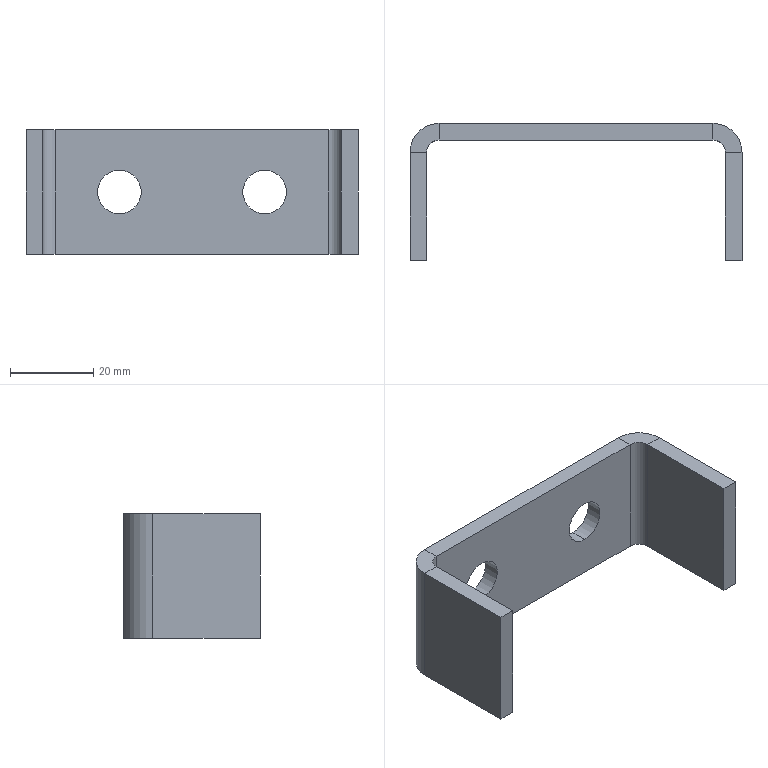Part | STEP file | SYL_0392D6J1SYL0380DJ10-1609202 | 1 solid | 26 faces | box 80 x 33 x 30 mm | volume 15352 mm3 | plane 18 | cylinder 8 | commonest cylinder face diameters 10.5 x4 6 x2 14 x2
STEP:
#1=CARTESIAN_POINT('',(-17.5,4.,5.25));
#2=VERTEX_POINT('',#1);
#3=CARTESIAN_POINT('',(-17.5,0.,5.25));
#4=VERTEX_POINT('',#3);
#5=CARTESIAN_POINT('',(-17.5,0.,5.25));
#6=DIRECTION('',(0.,-1.,0.));
#7=VECTOR('',#6,1000.);
#8=LINE('',#5,#7);
#9=EDGE_CURVE('',#2,#4,#8,.T.);
#10=ORIENTED_EDGE('',*,*,#9,.F.);
#11=CARTESIAN_POINT('',(-17.5,4.,-5.25));
#12=VERTEX_POINT('',#11);
#13=CARTESIAN_POINT('',(-17.5,4.,0.));
#14=DIRECTION('',(0.,1.,0.));
#15=DIRECTION('',(0.,0.,1.));
#16=AXIS2_PLACEMENT_3D('',#13,#14,#15);
#17=CIRCLE('',#16,5.25);
#18=EDGE_CURVE('',#2,#12,#17,.T.);
#19=ORIENTED_EDGE('',*,*,#18,.T.);
#20=CARTESIAN_POINT('',(-17.5,0.,-5.25));
#21=VERTEX_POINT('',#20);
#22=CARTESIAN_POINT('',(-17.5,0.,-5.25));
#23=DIRECTION('',(0.,-1.,0.));
#24=VECTOR('',#23,1000.);
#25=LINE('',#22,#24);
#26=EDGE_CURVE('',#12,#21,#25,.T.);
#27=ORIENTED_EDGE('',*,*,#26,.T.);
#28=CARTESIAN_POINT('',(-17.5,0.,0.));
#29=DIRECTION('',(0.,1.,0.));
#30=DIRECTION('',(0.,0.,1.));
#31=AXIS2_PLACEMENT_3D('',#28,#29,#30);
#32=CIRCLE('',#31,5.25);
#33=EDGE_CURVE('',#4,#21,#32,.T.);
#34=ORIENTED_EDGE('',*,*,#33,.F.);
#35=EDGE_LOOP('',(#10,#19,#27,#34));
#36=FACE_OUTER_BOUND('',#35,.T.);
#37=CARTESIAN_POINT('',(-17.5,0.,0.));
#38=DIRECTION('',(0.,1.,0.));
#39=DIRECTION('',(0.,0.,1.));
#40=AXIS2_PLACEMENT_3D('',#37,#38,#39);
#41=CYLINDRICAL_SURFACE('',#40,5.25);
#42=ADVANCED_FACE('',(#36),#41,.F.);
#43=CARTESIAN_POINT('',(17.5,4.,5.25));
#44=VERTEX_POINT('',#43);
#45=CARTESIAN_POINT('',(17.5,0.,5.25));
#46=VERTEX_POINT('',#45);
#47=CARTESIAN_POINT('',(17.5,0.,5.25));
#48=DIRECTION('',(0.,-1.,0.));
#49=VECTOR('',#48,1000.);
#50=LINE('',#47,#49);
#51=EDGE_CURVE('',#44,#46,#50,.T.);
#52=ORIENTED_EDGE('',*,*,#51,.F.);
#53=CARTESIAN_POINT('',(17.5,4.,-5.25));
#54=VERTEX_POINT('',#53);
#55=CARTESIAN_POINT('',(17.5,4.,0.));
#56=DIRECTION('',(0.,1.,0.));
#57=DIRECTION('',(0.,0.,1.));
#58=AXIS2_PLACEMENT_3D('',#55,#56,#57);
#59=CIRCLE('',#58,5.25);
#60=EDGE_CURVE('',#44,#54,#59,.T.);
#61=ORIENTED_EDGE('',*,*,#60,.T.);
#62=CARTESIAN_POINT('',(17.5,0.,-5.25));
#63=VERTEX_POINT('',#62);
#64=CARTESIAN_POINT('',(17.5,0.,-5.25));
#65=DIRECTION('',(0.,-1.,0.));
#66=VECTOR('',#65,1000.);
#67=LINE('',#64,#66);
#68=EDGE_CURVE('',#54,#63,#67,.T.);
#69=ORIENTED_EDGE('',*,*,#68,.T.);
#70=CARTESIAN_POINT('',(17.5,0.,0.));
#71=DIRECTION('',(0.,1.,0.));
#72=DIRECTION('',(0.,0.,1.));
#73=AXIS2_PLACEMENT_3D('',#70,#71,#72);
#74=CIRCLE('',#73,5.25);
#75=EDGE_CURVE('',#46,#63,#74,.T.);
#76=ORIENTED_EDGE('',*,*,#75,.F.);
#77=EDGE_LOOP('',(#52,#61,#69,#76));
#78=FACE_OUTER_BOUND('',#77,.T.);
#79=CARTESIAN_POINT('',(17.5,0.,0.));
#80=DIRECTION('',(0.,1.,0.));
#81=DIRECTION('',(0.,0.,1.));
#82=AXIS2_PLACEMENT_3D('',#79,#80,#81);
#83=CYLINDRICAL_SURFACE('',#82,5.25);
#84=ADVANCED_FACE('',(#78),#83,.F.);
#85=CARTESIAN_POINT('',(40.,-29.,-15.));
#86=VERTEX_POINT('',#85);
#87=CARTESIAN_POINT('',(36.,-29.,-15.));
#88=VERTEX_POINT('',#87);
#89=CARTESIAN_POINT('',(36.,-29.,-15.));
#90=DIRECTION('',(-1.,0.,0.));
#91=VECTOR('',#90,1000.);
#92=LINE('',#89,#91);
#93=EDGE_CURVE('',#86,#88,#92,.T.);
#94=ORIENTED_EDGE('',*,*,#93,.F.);
#95=CARTESIAN_POINT('',(40.,-29.,15.));
#96=VERTEX_POINT('',#95);
#97=CARTESIAN_POINT('',(40.,-29.,15.));
#98=DIRECTION('',(0.,0.,1.));
#99=VECTOR('',#98,1000.);
#100=LINE('',#97,#99);
#101=EDGE_CURVE('',#86,#96,#100,.T.);
#102=ORIENTED_EDGE('',*,*,#101,.T.);
#103=CARTESIAN_POINT('',(36.,-29.,15.));
#104=VERTEX_POINT('',#103);
#105=CARTESIAN_POINT('',(36.,-29.,15.));
#106=DIRECTION('',(-1.,0.,0.));
#107=VECTOR('',#106,1000.);
#108=LINE('',#105,#107);
#109=EDGE_CURVE('',#96,#104,#108,.T.);
#110=ORIENTED_EDGE('',*,*,#109,.T.);
#111=CARTESIAN_POINT('',(36.,-29.,-15.));
#112=DIRECTION('',(0.,0.,1.));
#113=VECTOR('',#112,1000.);
#114=LINE('',#111,#113);
#115=EDGE_CURVE('',#88,#104,#114,.T.);
#116=ORIENTED_EDGE('',*,*,#115,.F.);
#117=EDGE_LOOP('',(#94,#102,#110,#116));
#118=FACE_OUTER_BOUND('',#117,.T.);
#119=CARTESIAN_POINT('',(36.,-29.,-15.));
#120=DIRECTION('',(0.,1.,0.));
#121=DIRECTION('',(0.,0.,1.));
#122=AXIS2_PLACEMENT_3D('',#119,#120,#121);
#123=PLANE('',#122);
#124=ADVANCED_FACE('',(#118),#123,.F.);
#125=ORIENTED_EDGE('',*,*,#109,.F.);
#126=CARTESIAN_POINT('',(40.,-3.,15.));
#127=VERTEX_POINT('',#126);
#128=CARTESIAN_POINT('',(40.,4.,15.));
#129=DIRECTION('',(0.,1.,0.));
#130=VECTOR('',#129,1000.);
#131=LINE('',#128,#130);
#132=EDGE_CURVE('',#96,#127,#131,.T.);
#133=ORIENTED_EDGE('',*,*,#132,.T.);
#134=CARTESIAN_POINT('',(36.,-3.,15.));
#135=VERTEX_POINT('',#134);
#136=CARTESIAN_POINT('',(36.,-3.,15.));
#137=DIRECTION('',(-1.,0.,0.));
#138=VECTOR('',#137,1000.);
#139=LINE('',#136,#138);
#140=EDGE_CURVE('',#127,#135,#139,.T.);
#141=ORIENTED_EDGE('',*,*,#140,.T.);
#142=CARTESIAN_POINT('',(36.,-29.,15.));
#143=DIRECTION('',(0.,1.,0.));
#144=VECTOR('',#143,1000.);
#145=LINE('',#142,#144);
#146=EDGE_CURVE('',#104,#135,#145,.T.);
#147=ORIENTED_EDGE('',*,*,#146,.F.);
#148=EDGE_LOOP('',(#125,#133,#141,#147));
#149=FACE_OUTER_BOUND('',#148,.T.);
#150=CARTESIAN_POINT('',(36.,-29.,15.));
#151=DIRECTION('',(0.,0.,-1.));
#152=DIRECTION('',(0.,1.,0.));
#153=AXIS2_PLACEMENT_3D('',#150,#151,#152);
#154=PLANE('',#153);
#155=ADVANCED_FACE('',(#149),#154,.F.);
#156=ORIENTED_EDGE('',*,*,#140,.F.);
#157=CARTESIAN_POINT('',(33.,4.,15.));
#158=VERTEX_POINT('',#157);
#159=CARTESIAN_POINT('',(33.,-3.,15.));
#160=DIRECTION('',(0.,0.,-1.));
#161=DIRECTION('',(1.,0.,0.));
#162=AXIS2_PLACEMENT_3D('',#159,#160,#161);
#163=CIRCLE('',#162,7.);
#164=EDGE_CURVE('',#158,#127,#163,.T.);
#165=ORIENTED_EDGE('',*,*,#164,.F.);
#166=CARTESIAN_POINT('',(33.,0.,15.));
#167=VERTEX_POINT('',#166);
#168=CARTESIAN_POINT('',(33.,0.,15.));
#169=DIRECTION('',(0.,-1.,0.));
#170=VECTOR('',#169,1000.);
#171=LINE('',#168,#170);
#172=EDGE_CURVE('',#158,#167,#171,.T.);
#173=ORIENTED_EDGE('',*,*,#172,.T.);
#174=CARTESIAN_POINT('',(33.,-3.,15.));
#175=DIRECTION('',(0.,0.,-1.));
#176=DIRECTION('',(0.,1.,0.));
#177=AXIS2_PLACEMENT_3D('',#174,#175,#176);
#178=CIRCLE('',#177,3.);
#179=EDGE_CURVE('',#167,#135,#178,.T.);
#180=ORIENTED_EDGE('',*,*,#179,.T.);
#181=EDGE_LOOP('',(#156,#165,#173,#180));
#182=FACE_OUTER_BOUND('',#181,.T.);
#183=CARTESIAN_POINT('',(33.,-3.,15.));
#184=DIRECTION('',(0.,0.,1.));
#185=DIRECTION('',(1.,0.,0.));
#186=AXIS2_PLACEMENT_3D('',#183,#184,#185);
#187=PLANE('',#186);
#188=ADVANCED_FACE('',(#182),#187,.T.);
#189=ORIENTED_EDGE('',*,*,#172,.F.);
#190=CARTESIAN_POINT('',(-33.,4.,15.));
#191=VERTEX_POINT('',#190);
#192=CARTESIAN_POINT('',(0.,4.,15.));
#193=DIRECTION('',(-1.,0.,0.));
#194=VECTOR('',#193,1000.);
#195=LINE('',#192,#194);
#196=EDGE_CURVE('',#158,#191,#195,.T.);
#197=ORIENTED_EDGE('',*,*,#196,.T.);
#198=CARTESIAN_POINT('',(-33.,0.,15.));
#199=VERTEX_POINT('',#198);
#200=CARTESIAN_POINT('',(-33.,0.,15.));
#201=DIRECTION('',(0.,-1.,0.));
#202=VECTOR('',#201,1000.);
#203=LINE('',#200,#202);
#204=EDGE_CURVE('',#191,#199,#203,.T.);
#205=ORIENTED_EDGE('',*,*,#204,.T.);
#206=CARTESIAN_POINT('',(33.,0.,15.));
#207=DIRECTION('',(-1.,0.,0.));
#208=VECTOR('',#207,1000.);
#209=LINE('',#206,#208);
#210=EDGE_CURVE('',#167,#199,#209,.T.);
#211=ORIENTED_EDGE('',*,*,#210,.F.);
#212=EDGE_LOOP('',(#189,#197,#205,#211));
#213=FACE_OUTER_BOUND('',#212,.T.);
#214=CARTESIAN_POINT('',(33.,0.,15.));
#215=DIRECTION('',(0.,0.,-1.));
#216=DIRECTION('',(-1.,0.,0.));
#217=AXIS2_PLACEMENT_3D('',#214,#215,#216);
#218=PLANE('',#217);
#219=ADVANCED_FACE('',(#213),#218,.F.);
#220=ORIENTED_EDGE('',*,*,#204,.F.);
#221=CARTESIAN_POINT('',(-40.,-3.,15.));
#222=VERTEX_POINT('',#221);
#223=CARTESIAN_POINT('',(-33.,-3.,15.));
#224=DIRECTION('',(0.,0.,-1.));
#225=DIRECTION('',(-1.,0.,0.));
#226=AXIS2_PLACEMENT_3D('',#223,#224,#225);
#227=CIRCLE('',#226,7.);
#228=EDGE_CURVE('',#222,#191,#227,.T.);
#229=ORIENTED_EDGE('',*,*,#228,.F.);
#230=CARTESIAN_POINT('',(-36.,-3.,15.));
#231=VERTEX_POINT('',#230);
#232=CARTESIAN_POINT('',(-36.,-3.,15.));
#233=DIRECTION('',(1.,0.,0.));
#234=VECTOR('',#233,1000.);
#235=LINE('',#232,#234);
#236=EDGE_CURVE('',#222,#231,#235,.T.);
#237=ORIENTED_EDGE('',*,*,#236,.T.);
#238=CARTESIAN_POINT('',(-33.,-3.,15.));
#239=DIRECTION('',(0.,0.,-1.));
#240=DIRECTION('',(-1.,0.,0.));
#241=AXIS2_PLACEMENT_3D('',#238,#239,#240);
#242=CIRCLE('',#241,3.);
#243=EDGE_CURVE('',#231,#199,#242,.T.);
#244=ORIENTED_EDGE('',*,*,#243,.T.);
#245=EDGE_LOOP('',(#220,#229,#237,#244));
#246=FACE_OUTER_BOUND('',#245,.T.);
#247=CARTESIAN_POINT('',(-33.,-3.,15.));
#248=DIRECTION('',(0.,0.,1.));
#249=DIRECTION('',(1.,0.,0.));
#250=AXIS2_PLACEMENT_3D('',#247,#248,#249);
#251=PLANE('',#250);
#252=ADVANCED_FACE('',(#246),#251,.T.);
#253=ORIENTED_EDGE('',*,*,#236,.F.);
#254=CARTESIAN_POINT('',(-40.,-29.,15.));
#255=VERTEX_POINT('',#254);
#256=CARTESIAN_POINT('',(-40.,4.,15.));
#257=DIRECTION('',(0.,-1.,0.));
#258=VECTOR('',#257,1000.);
#259=LINE('',#256,#258);
#260=EDGE_CURVE('',#222,#255,#259,.T.);
#261=ORIENTED_EDGE('',*,*,#260,.T.);
#262=CARTESIAN_POINT('',(-36.,-29.,15.));
#263=VERTEX_POINT('',#262);
#264=CARTESIAN_POINT('',(-36.,-29.,15.));
#265=DIRECTION('',(1.,0.,0.));
#266=VECTOR('',#265,1000.);
#267=LINE('',#264,#266);
#268=EDGE_CURVE('',#255,#263,#267,.T.);
#269=ORIENTED_EDGE('',*,*,#268,.T.);
#270=CARTESIAN_POINT('',(-36.,-3.,15.));
#271=DIRECTION('',(0.,-1.,0.));
#272=VECTOR('',#271,1000.);
#273=LINE('',#270,#272);
#274=EDGE_CURVE('',#231,#263,#273,.T.);
#275=ORIENTED_EDGE('',*,*,#274,.F.);
#276=EDGE_LOOP('',(#253,#261,#269,#275));
#277=FACE_OUTER_BOUND('',#276,.T.);
#278=CARTESIAN_POINT('',(-36.,-3.,15.));
#279=DIRECTION('',(0.,0.,-1.));
#280=DIRECTION('',(0.,-1.,0.));
#281=AXIS2_PLACEMENT_3D('',#278,#279,#280);
#282=PLANE('',#281);
#283=ADVANCED_FACE('',(#277),#282,.F.);
#284=ORIENTED_EDGE('',*,*,#268,.F.);
#285=CARTESIAN_POINT('',(-40.,-29.,-15.));
#286=VERTEX_POINT('',#285);
#287=CARTESIAN_POINT('',(-40.,-29.,-15.));
#288=DIRECTION('',(0.,0.,-1.));
#289=VECTOR('',#288,1000.);
#290=LINE('',#287,#289);
#291=EDGE_CURVE('',#255,#286,#290,.T.);
#292=ORIENTED_EDGE('',*,*,#291,.T.);
#293=CARTESIAN_POINT('',(-36.,-29.,-15.));
#294=VERTEX_POINT('',#293);
#295=CARTESIAN_POINT('',(-36.,-29.,-15.));
#296=DIRECTION('',(1.,0.,0.));
#297=VECTOR('',#296,1000.);
#298=LINE('',#295,#297);
#299=EDGE_CURVE('',#286,#294,#298,.T.);
#300=ORIENTED_EDGE('',*,*,#299,.T.);
#301=CARTESIAN_POINT('',(-36.,-29.,15.));
#302=DIRECTION('',(0.,0.,-1.));
#303=VECTOR('',#302,1000.);
#304=LINE('',#301,#303);
#305=EDGE_CURVE('',#263,#294,#304,.T.);
#306=ORIENTED_EDGE('',*,*,#305,.F.);
#307=EDGE_LOOP('',(#284,#292,#300,#306));
#308=FACE_OUTER_BOUND('',#307,.T.);
#309=CARTESIAN_POINT('',(-36.,-29.,15.));
#310=DIRECTION('',(0.,1.,0.));
#311=DIRECTION('',(0.,0.,-1.));
#312=AXIS2_PLACEMENT_3D('',#309,#310,#311);
#313=PLANE('',#312);
#314=ADVANCED_FACE('',(#308),#313,.F.);
#315=ORIENTED_EDGE('',*,*,#299,.F.);
#316=CARTESIAN_POINT('',(-40.,-3.,-15.));
#317=VERTEX_POINT('',#316);
#318=CARTESIAN_POINT('',(-40.,4.,-15.));
#319=DIRECTION('',(0.,1.,0.));
#320=VECTOR('',#319,1000.);
#321=LINE('',#318,#320);
#322=EDGE_CURVE('',#286,#317,#321,.T.);
#323=ORIENTED_EDGE('',*,*,#322,.T.);
#324=CARTESIAN_POINT('',(-36.,-3.,-15.));
#325=VERTEX_POINT('',#324);
#326=CARTESIAN_POINT('',(-36.,-3.,-15.));
#327=DIRECTION('',(1.,0.,0.));
#328=VECTOR('',#327,1000.);
#329=LINE('',#326,#328);
#330=EDGE_CURVE('',#317,#325,#329,.T.);
#331=ORIENTED_EDGE('',*,*,#330,.T.);
#332=CARTESIAN_POINT('',(-36.,-29.,-15.));
#333=DIRECTION('',(0.,1.,0.));
#334=VECTOR('',#333,1000.);
#335=LINE('',#332,#334);
#336=EDGE_CURVE('',#294,#325,#335,.T.);
#337=ORIENTED_EDGE('',*,*,#336,.F.);
#338=EDGE_LOOP('',(#315,#323,#331,#337));
#339=FACE_OUTER_BOUND('',#338,.T.);
#340=CARTESIAN_POINT('',(-36.,-29.,-15.));
#341=DIRECTION('',(0.,0.,1.));
#342=DIRECTION('',(0.,1.,0.));
#343=AXIS2_PLACEMENT_3D('',#340,#341,#342);
#344=PLANE('',#343);
#345=ADVANCED_FACE('',(#339),#344,.F.);
#346=ORIENTED_EDGE('',*,*,#330,.F.);
#347=CARTESIAN_POINT('',(-33.,4.,-15.));
#348=VERTEX_POINT('',#347);
#349=CARTESIAN_POINT('',(-33.,-3.,-15.));
#350=DIRECTION('',(0.,0.,1.));
#351=DIRECTION('',(-1.,0.,0.));
#352=AXIS2_PLACEMENT_3D('',#349,#350,#351);
#353=CIRCLE('',#352,7.);
#354=EDGE_CURVE('',#348,#317,#353,.T.);
#355=ORIENTED_EDGE('',*,*,#354,.F.);
#356=CARTESIAN_POINT('',(-33.,0.,-15.));
#357=VERTEX_POINT('',#356);
#358=CARTESIAN_POINT('',(-33.,0.,-15.));
#359=DIRECTION('',(0.,-1.,0.));
#360=VECTOR('',#359,1000.);
#361=LINE('',#358,#360);
#362=EDGE_CURVE('',#348,#357,#361,.T.);
#363=ORIENTED_EDGE('',*,*,#362,.T.);
#364=CARTESIAN_POINT('',(-33.,-3.,-15.));
#365=DIRECTION('',(0.,0.,1.));
#366=DIRECTION('',(0.,1.,0.));
#367=AXIS2_PLACEMENT_3D('',#364,#365,#366);
#368=CIRCLE('',#367,3.);
#369=EDGE_CURVE('',#357,#325,#368,.T.);
#370=ORIENTED_EDGE('',*,*,#369,.T.);
#371=EDGE_LOOP('',(#346,#355,#363,#370));
#372=FACE_OUTER_BOUND('',#371,.T.);
#373=CARTESIAN_POINT('',(-33.,-3.,-15.));
#374=DIRECTION('',(0.,0.,-1.));
#375=DIRECTION('',(-1.,0.,0.));
#376=AXIS2_PLACEMENT_3D('',#373,#374,#375);
#377=PLANE('',#376);
#378=ADVANCED_FACE('',(#372),#377,.T.);
#379=ORIENTED_EDGE('',*,*,#362,.F.);
#380=CARTESIAN_POINT('',(33.,4.,-15.));
#381=VERTEX_POINT('',#380);
#382=CARTESIAN_POINT('',(0.,4.,-15.));
#383=DIRECTION('',(1.,0.,0.));
#384=VECTOR('',#383,1000.);
#385=LINE('',#382,#384);
#386=EDGE_CURVE('',#348,#381,#385,.T.);
#387=ORIENTED_EDGE('',*,*,#386,.T.);
#388=CARTESIAN_POINT('',(33.,0.,-15.));
#389=VERTEX_POINT('',#388);
#390=CARTESIAN_POINT('',(33.,0.,-15.));
#391=DIRECTION('',(0.,-1.,0.));
#392=VECTOR('',#391,1000.);
#393=LINE('',#390,#392);
#394=EDGE_CURVE('',#381,#389,#393,.T.);
#395=ORIENTED_EDGE('',*,*,#394,.T.);
#396=CARTESIAN_POINT('',(-33.,0.,-15.));
#397=DIRECTION('',(1.,0.,0.));
#398=VECTOR('',#397,1000.);
#399=LINE('',#396,#398);
#400=EDGE_CURVE('',#357,#389,#399,.T.);
#401=ORIENTED_EDGE('',*,*,#400,.F.);
#402=EDGE_LOOP('',(#379,#387,#395,#401));
#403=FACE_OUTER_BOUND('',#402,.T.);
#404=CARTESIAN_POINT('',(-33.,0.,-15.));
#405=DIRECTION('',(0.,0.,1.));
#406=DIRECTION('',(1.,0.,0.));
#407=AXIS2_PLACEMENT_3D('',#404,#405,#406);
#408=PLANE('',#407);
#409=ADVANCED_FACE('',(#403),#408,.F.);
#410=ORIENTED_EDGE('',*,*,#394,.F.);
#411=CARTESIAN_POINT('',(40.,-3.,-15.));
#412=VERTEX_POINT('',#411);
#413=CARTESIAN_POINT('',(33.,-3.,-15.));
#414=DIRECTION('',(0.,0.,1.));
#415=DIRECTION('',(1.,0.,0.));
#416=AXIS2_PLACEMENT_3D('',#413,#414,#415);
#417=CIRCLE('',#416,7.);
#418=EDGE_CURVE('',#412,#381,#417,.T.);
#419=ORIENTED_EDGE('',*,*,#418,.F.);
#420=CARTESIAN_POINT('',(36.,-3.,-15.));
#421=VERTEX_POINT('',#420);
#422=CARTESIAN_POINT('',(36.,-3.,-15.));
#423=DIRECTION('',(-1.,0.,0.));
#424=VECTOR('',#423,1000.);
#425=LINE('',#422,#424);
#426=EDGE_CURVE('',#412,#421,#425,.T.);
#427=ORIENTED_EDGE('',*,*,#426,.T.);
#428=CARTESIAN_POINT('',(33.,-3.,-15.));
#429=DIRECTION('',(0.,0.,1.));
#430=DIRECTION('',(1.,0.,0.));
#431=AXIS2_PLACEMENT_3D('',#428,#429,#430);
#432=CIRCLE('',#431,3.);
#433=EDGE_CURVE('',#421,#389,#432,.T.);
#434=ORIENTED_EDGE('',*,*,#433,.T.);
#435=EDGE_LOOP('',(#410,#419,#427,#434));
#436=FACE_OUTER_BOUND('',#435,.T.);
#437=CARTESIAN_POINT('',(33.,-3.,-15.));
#438=DIRECTION('',(0.,0.,-1.));
#439=DIRECTION('',(-1.,0.,0.));
#440=AXIS2_PLACEMENT_3D('',#437,#438,#439);
#441=PLANE('',#440);
#442=ADVANCED_FACE('',(#436),#441,.T.);
#443=CARTESIAN_POINT('',(17.5,4.,0.));
#444=DIRECTION('',(0.,1.,0.));
#445=DIRECTION('',(0.,0.,1.));
#446=AXIS2_PLACEMENT_3D('',#443,#444,#445);
#447=CIRCLE('',#446,5.25);
#448=EDGE_CURVE('',#54,#44,#447,.T.);
#449=ORIENTED_EDGE('',*,*,#448,.T.);
#450=ORIENTED_EDGE('',*,*,#51,.T.);
#451=CARTESIAN_POINT('',(17.5,0.,0.));
#452=DIRECTION('',(0.,1.,0.));
#453=DIRECTION('',(0.,0.,-1.));
#454=AXIS2_PLACEMENT_3D('',#451,#452,#453);
#455=CIRCLE('',#454,5.25);
#456=EDGE_CURVE('',#63,#46,#455,.T.);
#457=ORIENTED_EDGE('',*,*,#456,.F.);
#458=ORIENTED_EDGE('',*,*,#68,.F.);
#459=EDGE_LOOP('',(#449,#450,#457,#458));
#460=FACE_OUTER_BOUND('',#459,.T.);
#461=CARTESIAN_POINT('',(17.5,0.,0.));
#462=DIRECTION('',(0.,1.,0.));
#463=DIRECTION('',(0.,0.,1.));
#464=AXIS2_PLACEMENT_3D('',#461,#462,#463);
#465=CYLINDRICAL_SURFACE('',#464,5.25);
#466=ADVANCED_FACE('',(#460),#465,.F.);
#467=CARTESIAN_POINT('',(-17.5,4.,0.));
#468=DIRECTION('',(0.,1.,0.));
#469=DIRECTION('',(0.,0.,1.));
#470=AXIS2_PLACEMENT_3D('',#467,#468,#469);
#471=CIRCLE('',#470,5.25);
#472=EDGE_CURVE('',#12,#2,#471,.T.);
#473=ORIENTED_EDGE('',*,*,#472,.T.);
#474=ORIENTED_EDGE('',*,*,#9,.T.);
#475=CARTESIAN_POINT('',(-17.5,0.,0.));
#476=DIRECTION('',(0.,1.,0.));
#477=DIRECTION('',(0.,0.,-1.));
#478=AXIS2_PLACEMENT_3D('',#475,#476,#477);
#479=CIRCLE('',#478,5.25);
#480=EDGE_CURVE('',#21,#4,#479,.T.);
#481=ORIENTED_EDGE('',*,*,#480,.F.);
#482=ORIENTED_EDGE('',*,*,#26,.F.);
#483=EDGE_LOOP('',(#473,#474,#481,#482));
#484=FACE_OUTER_BOUND('',#483,.T.);
#485=CARTESIAN_POINT('',(-17.5,0.,0.));
#486=DIRECTION('',(0.,1.,0.));
#487=DIRECTION('',(0.,0.,1.));
#488=AXIS2_PLACEMENT_3D('',#485,#486,#487);
#489=CYLINDRICAL_SURFACE('',#488,5.25);
#490=ADVANCED_FACE('',(#484),#489,.F.);
#491=CARTESIAN_POINT('',(40.,4.,-15.));
#492=DIRECTION('',(0.,-1.,0.));
#493=VECTOR('',#492,1000.);
#494=LINE('',#491,#493);
#495=EDGE_CURVE('',#412,#86,#494,.T.);
#496=ORIENTED_EDGE('',*,*,#495,.T.);
#497=ORIENTED_EDGE('',*,*,#93,.T.);
#498=CARTESIAN_POINT('',(36.,-3.,-15.));
#499=DIRECTION('',(0.,-1.,0.));
#500=VECTOR('',#499,1000.);
#501=LINE('',#498,#500);
#502=EDGE_CURVE('',#421,#88,#501,.T.);
#503=ORIENTED_EDGE('',*,*,#502,.F.);
#504=ORIENTED_EDGE('',*,*,#426,.F.);
#505=EDGE_LOOP('',(#496,#497,#503,#504));
#506=FACE_OUTER_BOUND('',#505,.T.);
#507=CARTESIAN_POINT('',(36.,-3.,-15.));
#508=DIRECTION('',(0.,0.,1.));
#509=DIRECTION('',(0.,-1.,0.));
#510=AXIS2_PLACEMENT_3D('',#507,#508,#509);
#511=PLANE('',#510);
#512=ADVANCED_FACE('',(#506),#511,.F.);
#513=ORIENTED_EDGE('',*,*,#433,.F.);
#514=CARTESIAN_POINT('',(36.,-3.,-15.));
#515=DIRECTION('',(0.,0.,1.));
#516=VECTOR('',#515,1000.);
#517=LINE('',#514,#516);
#518=EDGE_CURVE('',#421,#135,#517,.T.);
#519=ORIENTED_EDGE('',*,*,#518,.T.);
#520=ORIENTED_EDGE('',*,*,#179,.F.);
#521=CARTESIAN_POINT('',(33.,0.,15.));
#522=DIRECTION('',(0.,0.,-1.));
#523=VECTOR('',#522,1000.);
#524=LINE('',#521,#523);
#525=EDGE_CURVE('',#167,#389,#524,.T.);
#526=ORIENTED_EDGE('',*,*,#525,.T.);
#527=EDGE_LOOP('',(#513,#519,#520,#526));
#528=FACE_OUTER_BOUND('',#527,.T.);
#529=CARTESIAN_POINT('',(33.,-3.,-15.));
#530=DIRECTION('',(0.,0.,1.));
#531=DIRECTION('',(1.,0.,0.));
#532=AXIS2_PLACEMENT_3D('',#529,#530,#531);
#533=CYLINDRICAL_SURFACE('',#532,3.);
#534=ADVANCED_FACE('',(#528),#533,.F.);
#535=ORIENTED_EDGE('',*,*,#115,.T.);
#536=ORIENTED_EDGE('',*,*,#146,.T.);
#537=ORIENTED_EDGE('',*,*,#518,.F.);
#538=ORIENTED_EDGE('',*,*,#502,.T.);
#539=EDGE_LOOP('',(#535,#536,#537,#538));
#540=FACE_OUTER_BOUND('',#539,.T.);
#541=CARTESIAN_POINT('',(36.,4.,15.));
#542=DIRECTION('',(1.,0.,0.));
#543=DIRECTION('',(0.,1.,0.));
#544=AXIS2_PLACEMENT_3D('',#541,#542,#543);
#545=PLANE('',#544);
#546=ADVANCED_FACE('',(#540),#545,.F.);
#547=ORIENTED_EDGE('',*,*,#243,.F.);
#548=CARTESIAN_POINT('',(-36.,-3.,15.));
#549=DIRECTION('',(0.,0.,-1.));
#550=VECTOR('',#549,1000.);
#551=LINE('',#548,#550);
#552=EDGE_CURVE('',#231,#325,#551,.T.);
#553=ORIENTED_EDGE('',*,*,#552,.T.);
#554=ORIENTED_EDGE('',*,*,#369,.F.);
#555=CARTESIAN_POINT('',(-33.,0.,-15.));
#556=DIRECTION('',(0.,0.,1.));
#557=VECTOR('',#556,1000.);
#558=LINE('',#555,#557);
#559=EDGE_CURVE('',#357,#199,#558,.T.);
#560=ORIENTED_EDGE('',*,*,#559,.T.);
#561=EDGE_LOOP('',(#547,#553,#554,#560));
#562=FACE_OUTER_BOUND('',#561,.T.);
#563=CARTESIAN_POINT('',(-33.,-3.,15.));
#564=DIRECTION('',(0.,0.,-1.));
#565=DIRECTION('',(-1.,0.,0.));
#566=AXIS2_PLACEMENT_3D('',#563,#564,#565);
#567=CYLINDRICAL_SURFACE('',#566,3.);
#568=ADVANCED_FACE('',(#562),#567,.F.);
#569=ORIENTED_EDGE('',*,*,#75,.T.);
#570=ORIENTED_EDGE('',*,*,#456,.T.);
#571=EDGE_LOOP('',(#569,#570));
#572=FACE_BOUND('',#571,.T.);
#573=ORIENTED_EDGE('',*,*,#33,.T.);
#574=ORIENTED_EDGE('',*,*,#480,.T.);
#575=EDGE_LOOP('',(#573,#574));
#576=FACE_BOUND('',#575,.T.);
#577=ORIENTED_EDGE('',*,*,#559,.F.);
#578=ORIENTED_EDGE('',*,*,#400,.T.);
#579=ORIENTED_EDGE('',*,*,#525,.F.);
#580=ORIENTED_EDGE('',*,*,#210,.T.);
#581=EDGE_LOOP('',(#577,#578,#579,#580));
#582=FACE_OUTER_BOUND('',#581,.T.);
#583=CARTESIAN_POINT('',(0.,0.,0.));
#584=DIRECTION('',(0.,1.,0.));
#585=DIRECTION('',(1.,0.,0.));
#586=AXIS2_PLACEMENT_3D('',#583,#584,#585);
#587=PLANE('',#586);
#588=ADVANCED_FACE('',(#572,#576,#582),#587,.F.);
#589=ORIENTED_EDGE('',*,*,#305,.T.);
#590=ORIENTED_EDGE('',*,*,#336,.T.);
#591=ORIENTED_EDGE('',*,*,#552,.F.);
#592=ORIENTED_EDGE('',*,*,#274,.T.);
#593=EDGE_LOOP('',(#589,#590,#591,#592));
#594=FACE_OUTER_BOUND('',#593,.T.);
#595=CARTESIAN_POINT('',(-36.,4.,-15.));
#596=DIRECTION('',(-1.,0.,0.));
#597=DIRECTION('',(0.,0.,1.));
#598=AXIS2_PLACEMENT_3D('',#595,#596,#597);
#599=PLANE('',#598);
#600=ADVANCED_FACE('',(#594),#599,.F.);
#601=ORIENTED_EDGE('',*,*,#418,.T.);
#602=CARTESIAN_POINT('',(33.,4.,-15.));
#603=DIRECTION('',(0.,0.,-1.));
#604=VECTOR('',#603,1000.);
#605=LINE('',#602,#604);
#606=EDGE_CURVE('',#158,#381,#605,.T.);
#607=ORIENTED_EDGE('',*,*,#606,.F.);
#608=ORIENTED_EDGE('',*,*,#164,.T.);
#609=CARTESIAN_POINT('',(40.,-3.,-15.));
#610=DIRECTION('',(0.,0.,1.));
#611=VECTOR('',#610,1000.);
#612=LINE('',#609,#611);
#613=EDGE_CURVE('',#412,#127,#612,.T.);
#614=ORIENTED_EDGE('',*,*,#613,.F.);
#615=EDGE_LOOP('',(#601,#607,#608,#614));
#616=FACE_OUTER_BOUND('',#615,.T.);
#617=CARTESIAN_POINT('',(33.,-3.,-15.));
#618=DIRECTION('',(0.,0.,1.));
#619=DIRECTION('',(1.,0.,0.));
#620=AXIS2_PLACEMENT_3D('',#617,#618,#619);
#621=CYLINDRICAL_SURFACE('',#620,7.);
#622=ADVANCED_FACE('',(#616),#621,.T.);
#623=ORIENTED_EDGE('',*,*,#101,.F.);
#624=ORIENTED_EDGE('',*,*,#495,.F.);
#625=ORIENTED_EDGE('',*,*,#613,.T.);
#626=ORIENTED_EDGE('',*,*,#132,.F.);
#627=EDGE_LOOP('',(#623,#624,#625,#626));
#628=FACE_OUTER_BOUND('',#627,.T.);
#629=CARTESIAN_POINT('',(40.,4.,15.));
#630=DIRECTION('',(1.,0.,0.));
#631=DIRECTION('',(0.,1.,0.));
#632=AXIS2_PLACEMENT_3D('',#629,#630,#631);
#633=PLANE('',#632);
#634=ADVANCED_FACE('',(#628),#633,.T.);
#635=ORIENTED_EDGE('',*,*,#228,.T.);
#636=CARTESIAN_POINT('',(-33.,4.,15.));
#637=DIRECTION('',(0.,0.,1.));
#638=VECTOR('',#637,1000.);
#639=LINE('',#636,#638);
#640=EDGE_CURVE('',#348,#191,#639,.T.);
#641=ORIENTED_EDGE('',*,*,#640,.F.);
#642=ORIENTED_EDGE('',*,*,#354,.T.);
#643=CARTESIAN_POINT('',(-40.,-3.,15.));
#644=DIRECTION('',(0.,0.,-1.));
#645=VECTOR('',#644,1000.);
#646=LINE('',#643,#645);
#647=EDGE_CURVE('',#222,#317,#646,.T.);
#648=ORIENTED_EDGE('',*,*,#647,.F.);
#649=EDGE_LOOP('',(#635,#641,#642,#648));
#650=FACE_OUTER_BOUND('',#649,.T.);
#651=CARTESIAN_POINT('',(-33.,-3.,15.));
#652=DIRECTION('',(0.,0.,-1.));
#653=DIRECTION('',(-1.,0.,0.));
#654=AXIS2_PLACEMENT_3D('',#651,#652,#653);
#655=CYLINDRICAL_SURFACE('',#654,7.);
#656=ADVANCED_FACE('',(#650),#655,.T.);
#657=ORIENTED_EDGE('',*,*,#60,.F.);
#658=ORIENTED_EDGE('',*,*,#448,.F.);
#659=EDGE_LOOP('',(#657,#658));
#660=FACE_BOUND('',#659,.T.);
#661=ORIENTED_EDGE('',*,*,#18,.F.);
#662=ORIENTED_EDGE('',*,*,#472,.F.);
#663=EDGE_LOOP('',(#661,#662));
#664=FACE_BOUND('',#663,.T.);
#665=ORIENTED_EDGE('',*,*,#640,.T.);
#666=ORIENTED_EDGE('',*,*,#196,.F.);
#667=ORIENTED_EDGE('',*,*,#606,.T.);
#668=ORIENTED_EDGE('',*,*,#386,.F.);
#669=EDGE_LOOP('',(#665,#666,#667,#668));
#670=FACE_OUTER_BOUND('',#669,.T.);
#671=CARTESIAN_POINT('',(0.,4.,0.));
#672=DIRECTION('',(0.,1.,0.));
#673=DIRECTION('',(1.,0.,0.));
#674=AXIS2_PLACEMENT_3D('',#671,#672,#673);
#675=PLANE('',#674);
#676=ADVANCED_FACE('',(#660,#664,#670),#675,.T.);
#677=ORIENTED_EDGE('',*,*,#291,.F.);
#678=ORIENTED_EDGE('',*,*,#260,.F.);
#679=ORIENTED_EDGE('',*,*,#647,.T.);
#680=ORIENTED_EDGE('',*,*,#322,.F.);
#681=EDGE_LOOP('',(#677,#678,#679,#680));
#682=FACE_OUTER_BOUND('',#681,.T.);
#683=CARTESIAN_POINT('',(-40.,4.,-15.));
#684=DIRECTION('',(-1.,0.,0.));
#685=DIRECTION('',(0.,0.,1.));
#686=AXIS2_PLACEMENT_3D('',#683,#684,#685);
#687=PLANE('',#686);
#688=ADVANCED_FACE('',(#682),#687,.T.);
#689=CLOSED_SHELL('',(#42,#84,#124,#155,#188,#219,#252,#283,#314,#345,#378,#409,#442,#466,#490,#512,#534,#546,#568,#588,#600,#622,#634,#656,#676,#688));
#690=MANIFOLD_SOLID_BREP('',#689);
#691=CARTESIAN_POINT('',(0.,0.,0.));
#692=DIRECTION('',(0.,0.,1.));
#693=DIRECTION('',(1.,0.,0.));
#694=AXIS2_PLACEMENT_3D('',#691,#692,#693);
#695=(LENGTH_UNIT()NAMED_UNIT(*)SI_UNIT(.MILLI.,.METRE.));
#696=UNCERTAINTY_MEASURE_WITH_UNIT(LENGTH_MEASURE(0.00001),#695,'','');
#697=(NAMED_UNIT(*)PLANE_ANGLE_UNIT()SI_UNIT($,.RADIAN.));
#698=(NAMED_UNIT(*)SI_UNIT($,.STERADIAN.)SOLID_ANGLE_UNIT());
#699=(GEOMETRIC_REPRESENTATION_CONTEXT(3)GLOBAL_UNCERTAINTY_ASSIGNED_CONTEXT((#696))GLOBAL_UNIT_ASSIGNED_CONTEXT((#695,#697,#698))REPRESENTATION_CONTEXT('',''));
#700=ADVANCED_BREP_SHAPE_REPRESENTATION('',(#690,#694),#699);